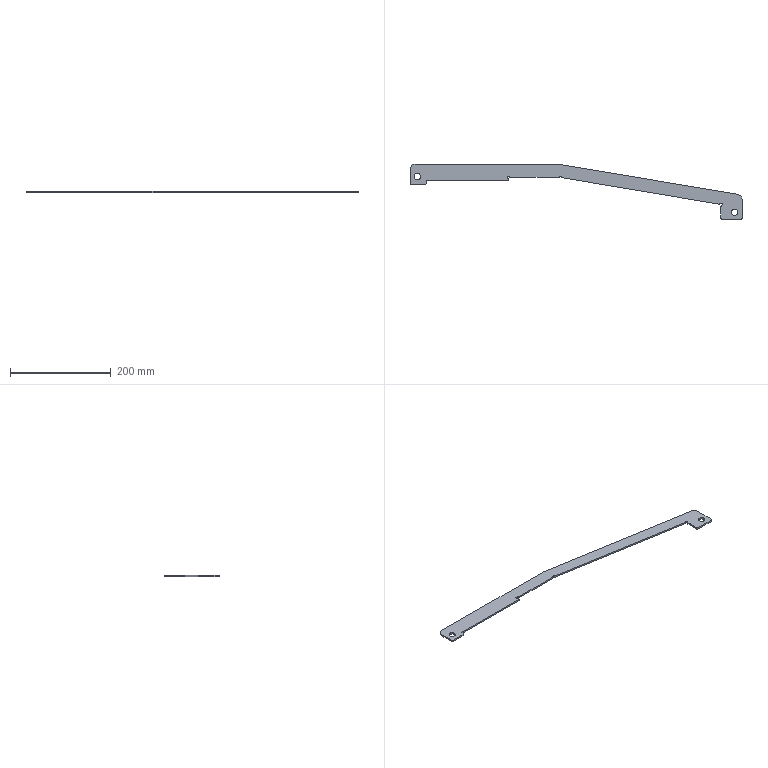Part | SolidWorks | features Fillet 2, FlatPattern 1, SMBaseFlange 1, SheetMetal 1 | 1 solid | 34 faces | box 659 x 110.2 x 3 mm | volume 58163 mm3 | cylinder 20 | plane 14 | commonest cylinder face diameters 4 x6 5 x4 6 x4 12.5 x4 20 x2
STEP:
#1=CARTESIAN_POINT('',(-277.647,51.799,3.));
#2=VERTEX_POINT('',#1);
#3=CARTESIAN_POINT('',(-265.147,51.799,3.));
#4=VERTEX_POINT('',#3);
#5=CARTESIAN_POINT('',(-271.397,51.799,3.));
#6=DIRECTION('',(0.,0.,1.));
#7=DIRECTION('',(1.,0.,0.));
#8=AXIS2_PLACEMENT_3D('',#5,#6,#7);
#9=CIRCLE('',#8,6.25);
#10=EDGE_CURVE('',#2,#4,#9,.T.);
#11=ORIENTED_EDGE('',*,*,#10,.T.);
#12=CARTESIAN_POINT('',(-265.147,51.799,0.));
#13=VERTEX_POINT('',#12);
#14=CARTESIAN_POINT('',(-265.147,51.799,3.));
#15=DIRECTION('',(0.,0.,-1.));
#16=VECTOR('',#15,1000.);
#17=LINE('',#14,#16);
#18=EDGE_CURVE('',#4,#13,#17,.T.);
#19=ORIENTED_EDGE('',*,*,#18,.T.);
#20=CARTESIAN_POINT('',(-277.647,51.799,0.));
#21=VERTEX_POINT('',#20);
#22=CARTESIAN_POINT('',(-271.397,51.799,0.));
#23=DIRECTION('',(0.,0.,1.));
#24=DIRECTION('',(1.,0.,0.));
#25=AXIS2_PLACEMENT_3D('',#22,#23,#24);
#26=CIRCLE('',#25,6.25);
#27=EDGE_CURVE('',#21,#13,#26,.T.);
#28=ORIENTED_EDGE('',*,*,#27,.F.);
#29=CARTESIAN_POINT('',(-277.647,51.799,3.));
#30=DIRECTION('',(0.,0.,-1.));
#31=VECTOR('',#30,1000.);
#32=LINE('',#29,#31);
#33=EDGE_CURVE('',#2,#21,#32,.T.);
#34=ORIENTED_EDGE('',*,*,#33,.F.);
#35=EDGE_LOOP('',(#11,#19,#28,#34));
#36=FACE_OUTER_BOUND('',#35,.T.);
#37=CARTESIAN_POINT('',(-271.397,51.799,3.));
#38=DIRECTION('',(0.,0.,-1.));
#39=DIRECTION('',(-1.,0.,0.));
#40=AXIS2_PLACEMENT_3D('',#37,#38,#39);
#41=CYLINDRICAL_SURFACE('',#40,6.25);
#42=ADVANCED_FACE('',(#36),#41,.F.);
#43=CARTESIAN_POINT('',(352.353,-18.901,3.));
#44=VERTEX_POINT('',#43);
#45=CARTESIAN_POINT('',(364.853,-18.901,3.));
#46=VERTEX_POINT('',#45);
#47=CARTESIAN_POINT('',(358.603,-18.901,3.));
#48=DIRECTION('',(0.,0.,1.));
#49=DIRECTION('',(1.,0.,0.));
#50=AXIS2_PLACEMENT_3D('',#47,#48,#49);
#51=CIRCLE('',#50,6.25);
#52=EDGE_CURVE('',#44,#46,#51,.T.);
#53=ORIENTED_EDGE('',*,*,#52,.T.);
#54=CARTESIAN_POINT('',(364.853,-18.901,0.));
#55=VERTEX_POINT('',#54);
#56=CARTESIAN_POINT('',(364.853,-18.901,3.));
#57=DIRECTION('',(0.,0.,-1.));
#58=VECTOR('',#57,1000.);
#59=LINE('',#56,#58);
#60=EDGE_CURVE('',#46,#55,#59,.T.);
#61=ORIENTED_EDGE('',*,*,#60,.T.);
#62=CARTESIAN_POINT('',(352.353,-18.901,0.));
#63=VERTEX_POINT('',#62);
#64=CARTESIAN_POINT('',(358.603,-18.901,0.));
#65=DIRECTION('',(0.,0.,1.));
#66=DIRECTION('',(1.,0.,0.));
#67=AXIS2_PLACEMENT_3D('',#64,#65,#66);
#68=CIRCLE('',#67,6.25);
#69=EDGE_CURVE('',#63,#55,#68,.T.);
#70=ORIENTED_EDGE('',*,*,#69,.F.);
#71=CARTESIAN_POINT('',(352.353,-18.901,3.));
#72=DIRECTION('',(0.,0.,-1.));
#73=VECTOR('',#72,1000.);
#74=LINE('',#71,#73);
#75=EDGE_CURVE('',#44,#63,#74,.T.);
#76=ORIENTED_EDGE('',*,*,#75,.F.);
#77=EDGE_LOOP('',(#53,#61,#70,#76));
#78=FACE_OUTER_BOUND('',#77,.T.);
#79=CARTESIAN_POINT('',(358.603,-18.901,3.));
#80=DIRECTION('',(0.,0.,-1.));
#81=DIRECTION('',(-1.,0.,0.));
#82=AXIS2_PLACEMENT_3D('',#79,#80,#81);
#83=CYLINDRICAL_SURFACE('',#82,6.25);
#84=ADVANCED_FACE('',(#78),#83,.F.);
#85=CARTESIAN_POINT('',(-92.897,50.099,3.));
#86=VERTEX_POINT('',#85);
#87=CARTESIAN_POINT('',(-88.157,51.21,3.));
#88=VERTEX_POINT('',#87);
#89=CARTESIAN_POINT('',(-90.397,50.099,3.));
#90=DIRECTION('',(0.,0.,-1.));
#91=DIRECTION('',(1.,0.,0.));
#92=AXIS2_PLACEMENT_3D('',#89,#90,#91);
#93=CIRCLE('',#92,2.5);
#94=EDGE_CURVE('',#86,#88,#93,.T.);
#95=ORIENTED_EDGE('',*,*,#94,.F.);
#96=CARTESIAN_POINT('',(-92.897,50.099,0.));
#97=VERTEX_POINT('',#96);
#98=CARTESIAN_POINT('',(-92.897,50.099,3.));
#99=DIRECTION('',(0.,0.,-1.));
#100=VECTOR('',#99,1000.);
#101=LINE('',#98,#100);
#102=EDGE_CURVE('',#86,#97,#101,.T.);
#103=ORIENTED_EDGE('',*,*,#102,.T.);
#104=CARTESIAN_POINT('',(-88.157,51.21,0.));
#105=VERTEX_POINT('',#104);
#106=CARTESIAN_POINT('',(-90.397,50.099,0.));
#107=DIRECTION('',(0.,0.,-1.));
#108=DIRECTION('',(1.,0.,0.));
#109=AXIS2_PLACEMENT_3D('',#106,#107,#108);
#110=CIRCLE('',#109,2.5);
#111=EDGE_CURVE('',#97,#105,#110,.T.);
#112=ORIENTED_EDGE('',*,*,#111,.T.);
#113=CARTESIAN_POINT('',(-88.157,51.21,3.));
#114=DIRECTION('',(0.,0.,1.));
#115=VECTOR('',#114,1000.);
#116=LINE('',#113,#115);
#117=EDGE_CURVE('',#105,#88,#116,.T.);
#118=ORIENTED_EDGE('',*,*,#117,.T.);
#119=EDGE_LOOP('',(#95,#103,#112,#118));
#120=FACE_OUTER_BOUND('',#119,.T.);
#121=CARTESIAN_POINT('',(-90.397,50.099,3.));
#122=DIRECTION('',(0.,0.,-1.));
#123=DIRECTION('',(-1.,0.,0.));
#124=AXIS2_PLACEMENT_3D('',#121,#122,#123);
#125=CYLINDRICAL_SURFACE('',#124,2.5);
#126=ADVANCED_FACE('',(#120),#125,.F.);
#127=CARTESIAN_POINT('',(-90.397,43.499,3.));
#128=VERTEX_POINT('',#127);
#129=CARTESIAN_POINT('',(-90.397,46.068,3.));
#130=VERTEX_POINT('',#129);
#131=CARTESIAN_POINT('',(-90.397,47.599,3.));
#132=DIRECTION('',(0.,1.,0.));
#133=VECTOR('',#132,1000.);
#134=LINE('',#131,#133);
#135=EDGE_CURVE('',#128,#130,#134,.T.);
#136=ORIENTED_EDGE('',*,*,#135,.T.);
#137=CARTESIAN_POINT('',(-91.508,47.86,3.));
#138=VERTEX_POINT('',#137);
#139=CARTESIAN_POINT('',(-92.397,46.068,3.));
#140=DIRECTION('',(0.,0.,1.));
#141=DIRECTION('',(-1.,0.,0.));
#142=AXIS2_PLACEMENT_3D('',#139,#140,#141);
#143=CIRCLE('',#142,2.);
#144=EDGE_CURVE('',#130,#138,#143,.T.);
#145=ORIENTED_EDGE('',*,*,#144,.T.);
#146=CARTESIAN_POINT('',(-90.397,50.099,3.));
#147=DIRECTION('',(0.,0.,-1.));
#148=DIRECTION('',(1.,0.,0.));
#149=AXIS2_PLACEMENT_3D('',#146,#147,#148);
#150=CIRCLE('',#149,2.5);
#151=EDGE_CURVE('',#138,#86,#150,.T.);
#152=ORIENTED_EDGE('',*,*,#151,.T.);
#153=ORIENTED_EDGE('',*,*,#94,.T.);
#154=CARTESIAN_POINT('',(-86.365,50.099,3.));
#155=VERTEX_POINT('',#154);
#156=CARTESIAN_POINT('',(-86.365,52.099,3.));
#157=DIRECTION('',(0.,0.,1.));
#158=DIRECTION('',(-1.,0.,0.));
#159=AXIS2_PLACEMENT_3D('',#156,#157,#158);
#160=CIRCLE('',#159,2.);
#161=EDGE_CURVE('',#88,#155,#160,.T.);
#162=ORIENTED_EDGE('',*,*,#161,.T.);
#163=CARTESIAN_POINT('',(8.706,50.099,3.));
#164=VERTEX_POINT('',#163);
#165=CARTESIAN_POINT('',(10.237,50.099,3.));
#166=DIRECTION('',(1.,-0.000000002,0.));
#167=VECTOR('',#166,1000.);
#168=LINE('',#165,#167);
#169=EDGE_CURVE('',#155,#164,#168,.T.);
#170=ORIENTED_EDGE('',*,*,#169,.T.);
#171=CARTESIAN_POINT('',(10.497,51.21,3.));
#172=VERTEX_POINT('',#171);
#173=CARTESIAN_POINT('',(8.706,52.099,3.));
#174=DIRECTION('',(0.,0.,1.));
#175=DIRECTION('',(-1.,0.,0.));
#176=AXIS2_PLACEMENT_3D('',#173,#174,#175);
#177=CIRCLE('',#176,2.);
#178=EDGE_CURVE('',#164,#172,#177,.T.);
#179=ORIENTED_EDGE('',*,*,#178,.T.);
#180=CARTESIAN_POINT('',(15.13,50.824,3.));
#181=VERTEX_POINT('',#180);
#182=CARTESIAN_POINT('',(12.737,50.099,3.));
#183=DIRECTION('',(0.,0.,-1.));
#184=DIRECTION('',(1.,0.,0.));
#185=AXIS2_PLACEMENT_3D('',#182,#183,#184);
#186=CIRCLE('',#185,2.5);
#187=EDGE_CURVE('',#172,#181,#186,.T.);
#188=ORIENTED_EDGE('',*,*,#187,.T.);
#189=CARTESIAN_POINT('',(16.712,49.431,3.));
#190=VERTEX_POINT('',#189);
#191=CARTESIAN_POINT('',(17.044,51.403,3.));
#192=DIRECTION('',(0.,0.,1.));
#193=DIRECTION('',(-1.,0.,0.));
#194=AXIS2_PLACEMENT_3D('',#191,#192,#193);
#195=CIRCLE('',#194,2.);
#196=EDGE_CURVE('',#181,#190,#195,.T.);
#197=ORIENTED_EDGE('',*,*,#196,.T.);
#198=CARTESIAN_POINT('',(327.328,-2.779,3.));
#199=VERTEX_POINT('',#198);
#200=CARTESIAN_POINT('',(328.838,-3.033,3.));
#201=DIRECTION('',(0.9862,-0.1658,0.));
#202=VECTOR('',#201,1000.);
#203=LINE('',#200,#202);
#204=EDGE_CURVE('',#190,#199,#203,.T.);
#205=ORIENTED_EDGE('',*,*,#204,.T.);
#206=CARTESIAN_POINT('',(329.279,-1.98,3.));
#207=VERTEX_POINT('',#206);
#208=CARTESIAN_POINT('',(327.66,-0.8068,3.));
#209=DIRECTION('',(0.,0.,1.));
#210=DIRECTION('',(-1.,0.,0.));
#211=AXIS2_PLACEMENT_3D('',#208,#209,#210);
#212=CIRCLE('',#211,2.);
#213=EDGE_CURVE('',#199,#207,#212,.T.);
#214=ORIENTED_EDGE('',*,*,#213,.T.);
#215=CARTESIAN_POINT('',(332.415,-5.687,3.));
#216=VERTEX_POINT('',#215);
#217=CARTESIAN_POINT('',(331.303,-3.447,3.));
#218=DIRECTION('',(0.,0.,-1.));
#219=DIRECTION('',(1.,0.,0.));
#220=AXIS2_PLACEMENT_3D('',#217,#218,#219);
#221=CIRCLE('',#220,2.5);
#222=EDGE_CURVE('',#207,#216,#221,.T.);
#223=ORIENTED_EDGE('',*,*,#222,.T.);
#224=CARTESIAN_POINT('',(331.303,-7.478,3.));
#225=VERTEX_POINT('',#224);
#226=CARTESIAN_POINT('',(333.303,-7.478,3.));
#227=DIRECTION('',(0.,0.,1.));
#228=DIRECTION('',(-1.,0.,0.));
#229=AXIS2_PLACEMENT_3D('',#226,#227,#228);
#230=CIRCLE('',#229,2.);
#231=EDGE_CURVE('',#216,#225,#230,.T.);
#232=ORIENTED_EDGE('',*,*,#231,.T.);
#233=CARTESIAN_POINT('',(331.303,-30.901,3.));
#234=VERTEX_POINT('',#233);
#235=CARTESIAN_POINT('',(331.303,-33.901,3.));
#236=DIRECTION('',(0.,-1.,0.));
#237=VECTOR('',#236,1000.);
#238=LINE('',#235,#237);
#239=EDGE_CURVE('',#225,#234,#238,.T.);
#240=ORIENTED_EDGE('',*,*,#239,.T.);
#241=CARTESIAN_POINT('',(334.303,-33.901,3.));
#242=VERTEX_POINT('',#241);
#243=CARTESIAN_POINT('',(334.303,-30.901,3.));
#244=DIRECTION('',(0.,0.,1.));
#245=DIRECTION('',(-1.,0.,0.));
#246=AXIS2_PLACEMENT_3D('',#243,#244,#245);
#247=CIRCLE('',#246,3.);
#248=EDGE_CURVE('',#234,#242,#247,.T.);
#249=ORIENTED_EDGE('',*,*,#248,.T.);
#250=CARTESIAN_POINT('',(370.103,-33.901,3.));
#251=VERTEX_POINT('',#250);
#252=CARTESIAN_POINT('',(331.303,-33.901,3.));
#253=DIRECTION('',(1.,0.,0.));
#254=VECTOR('',#253,1000.);
#255=LINE('',#252,#254);
#256=EDGE_CURVE('',#242,#251,#255,.T.);
#257=ORIENTED_EDGE('',*,*,#256,.T.);
#258=CARTESIAN_POINT('',(373.103,-30.901,3.));
#259=VERTEX_POINT('',#258);
#260=CARTESIAN_POINT('',(370.103,-30.901,3.));
#261=DIRECTION('',(0.,0.,1.));
#262=DIRECTION('',(-1.,0.,0.));
#263=AXIS2_PLACEMENT_3D('',#260,#261,#262);
#264=CIRCLE('',#263,3.);
#265=EDGE_CURVE('',#251,#259,#264,.T.);
#266=ORIENTED_EDGE('',*,*,#265,.T.);
#267=CARTESIAN_POINT('',(373.103,6.871,3.));
#268=VERTEX_POINT('',#267);
#269=CARTESIAN_POINT('',(373.103,-33.901,3.));
#270=DIRECTION('',(0.,1.,0.));
#271=VECTOR('',#270,1000.);
#272=LINE('',#269,#271);
#273=EDGE_CURVE('',#259,#268,#272,.T.);
#274=ORIENTED_EDGE('',*,*,#273,.T.);
#275=CARTESIAN_POINT('',(364.753,16.734,3.));
#276=VERTEX_POINT('',#275);
#277=CARTESIAN_POINT('',(363.103,6.871,3.));
#278=DIRECTION('',(0.,0.,1.));
#279=DIRECTION('',(-1.,0.,0.));
#280=AXIS2_PLACEMENT_3D('',#277,#278,#279);
#281=CIRCLE('',#280,10.);
#282=EDGE_CURVE('',#268,#276,#281,.T.);
#283=ORIENTED_EDGE('',*,*,#282,.T.);
#284=CARTESIAN_POINT('',(8.534,76.299,3.));
#285=VERTEX_POINT('',#284);
#286=CARTESIAN_POINT('',(364.753,16.734,3.));
#287=DIRECTION('',(-0.9863,0.1649,0.));
#288=VECTOR('',#287,1000.);
#289=LINE('',#286,#288);
#290=EDGE_CURVE('',#276,#285,#289,.T.);
#291=ORIENTED_EDGE('',*,*,#290,.T.);
#292=CARTESIAN_POINT('',(-275.897,76.299,3.));
#293=VERTEX_POINT('',#292);
#294=CARTESIAN_POINT('',(-275.897,76.299,3.));
#295=DIRECTION('',(-1.,0.,0.));
#296=VECTOR('',#295,1000.);
#297=LINE('',#294,#296);
#298=EDGE_CURVE('',#285,#293,#297,.T.);
#299=ORIENTED_EDGE('',*,*,#298,.T.);
#300=CARTESIAN_POINT('',(-285.897,66.299,3.));
#301=VERTEX_POINT('',#300);
#302=CARTESIAN_POINT('',(-275.897,66.299,3.));
#303=DIRECTION('',(0.,0.,1.));
#304=DIRECTION('',(-1.,0.,0.));
#305=AXIS2_PLACEMENT_3D('',#302,#303,#304);
#306=CIRCLE('',#305,10.);
#307=EDGE_CURVE('',#293,#301,#306,.T.);
#308=ORIENTED_EDGE('',*,*,#307,.T.);
#309=CARTESIAN_POINT('',(-285.897,39.299,3.));
#310=VERTEX_POINT('',#309);
#311=CARTESIAN_POINT('',(-285.897,36.299,3.));
#312=DIRECTION('',(0.,-1.,0.));
#313=VECTOR('',#312,1000.);
#314=LINE('',#311,#313);
#315=EDGE_CURVE('',#301,#310,#314,.T.);
#316=ORIENTED_EDGE('',*,*,#315,.T.);
#317=CARTESIAN_POINT('',(-282.897,36.299,3.));
#318=VERTEX_POINT('',#317);
#319=CARTESIAN_POINT('',(-282.897,39.299,3.));
#320=DIRECTION('',(0.,0.,1.));
#321=DIRECTION('',(-1.,0.,0.));
#322=AXIS2_PLACEMENT_3D('',#319,#320,#321);
#323=CIRCLE('',#322,3.);
#324=EDGE_CURVE('',#310,#318,#323,.T.);
#325=ORIENTED_EDGE('',*,*,#324,.T.);
#326=CARTESIAN_POINT('',(-256.397,36.299,3.));
#327=VERTEX_POINT('',#326);
#328=CARTESIAN_POINT('',(-253.397,36.299,3.));
#329=DIRECTION('',(1.,0.,0.));
#330=VECTOR('',#329,1000.);
#331=LINE('',#328,#330);
#332=EDGE_CURVE('',#318,#327,#331,.T.);
#333=ORIENTED_EDGE('',*,*,#332,.T.);
#334=CARTESIAN_POINT('',(-253.397,39.299,3.));
#335=VERTEX_POINT('',#334);
#336=CARTESIAN_POINT('',(-256.397,39.299,3.));
#337=DIRECTION('',(0.,0.,1.));
#338=DIRECTION('',(-1.,0.,0.));
#339=AXIS2_PLACEMENT_3D('',#336,#337,#338);
#340=CIRCLE('',#339,3.);
#341=EDGE_CURVE('',#327,#335,#340,.T.);
#342=ORIENTED_EDGE('',*,*,#341,.T.);
#343=CARTESIAN_POINT('',(-253.397,43.499,3.));
#344=VERTEX_POINT('',#343);
#345=CARTESIAN_POINT('',(-253.397,43.499,3.));
#346=DIRECTION('',(0.,1.,0.));
#347=VECTOR('',#346,1000.);
#348=LINE('',#345,#347);
#349=EDGE_CURVE('',#335,#344,#348,.T.);
#350=ORIENTED_EDGE('',*,*,#349,.T.);
#351=CARTESIAN_POINT('',(-90.397,43.499,3.));
#352=DIRECTION('',(1.,0.,0.));
#353=VECTOR('',#352,1000.);
#354=LINE('',#351,#353);
#355=EDGE_CURVE('',#344,#128,#354,.T.);
#356=ORIENTED_EDGE('',*,*,#355,.T.);
#357=EDGE_LOOP('',(#136,#145,#152,#153,#162,#170,#179,#188,#197,#205,#214,#223,#232,#240,#249,#257,#266,#274,#283,#291,#299,#308,#316,#325,#333,#342,#350,#356));
#358=FACE_OUTER_BOUND('',#357,.T.);
#359=ORIENTED_EDGE('',*,*,#52,.F.);
#360=CARTESIAN_POINT('',(358.603,-18.901,3.));
#361=DIRECTION('',(0.,0.,1.));
#362=DIRECTION('',(1.,0.,0.));
#363=AXIS2_PLACEMENT_3D('',#360,#361,#362);
#364=CIRCLE('',#363,6.25);
#365=EDGE_CURVE('',#46,#44,#364,.T.);
#366=ORIENTED_EDGE('',*,*,#365,.F.);
#367=EDGE_LOOP('',(#359,#366));
#368=FACE_BOUND('',#367,.T.);
#369=ORIENTED_EDGE('',*,*,#10,.F.);
#370=CARTESIAN_POINT('',(-271.397,51.799,3.));
#371=DIRECTION('',(0.,0.,1.));
#372=DIRECTION('',(1.,0.,0.));
#373=AXIS2_PLACEMENT_3D('',#370,#371,#372);
#374=CIRCLE('',#373,6.25);
#375=EDGE_CURVE('',#4,#2,#374,.T.);
#376=ORIENTED_EDGE('',*,*,#375,.F.);
#377=EDGE_LOOP('',(#369,#376));
#378=FACE_BOUND('',#377,.T.);
#379=CARTESIAN_POINT('',(-275.897,66.299,3.));
#380=DIRECTION('',(0.,0.,-1.));
#381=DIRECTION('',(-1.,0.,0.));
#382=AXIS2_PLACEMENT_3D('',#379,#380,#381);
#383=PLANE('',#382);
#384=ADVANCED_FACE('',(#358,#368,#378),#383,.F.);
#385=ORIENTED_EDGE('',*,*,#69,.T.);
#386=CARTESIAN_POINT('',(358.603,-18.901,0.));
#387=DIRECTION('',(0.,0.,1.));
#388=DIRECTION('',(1.,0.,0.));
#389=AXIS2_PLACEMENT_3D('',#386,#387,#388);
#390=CIRCLE('',#389,6.25);
#391=EDGE_CURVE('',#55,#63,#390,.T.);
#392=ORIENTED_EDGE('',*,*,#391,.T.);
#393=EDGE_LOOP('',(#385,#392));
#394=FACE_BOUND('',#393,.T.);
#395=CARTESIAN_POINT('',(-91.508,47.86,0.));
#396=VERTEX_POINT('',#395);
#397=CARTESIAN_POINT('',(-90.397,50.099,0.));
#398=DIRECTION('',(0.,0.,-1.));
#399=DIRECTION('',(1.,0.,0.));
#400=AXIS2_PLACEMENT_3D('',#397,#398,#399);
#401=CIRCLE('',#400,2.5);
#402=EDGE_CURVE('',#396,#97,#401,.T.);
#403=ORIENTED_EDGE('',*,*,#402,.F.);
#404=CARTESIAN_POINT('',(-90.397,46.068,0.));
#405=VERTEX_POINT('',#404);
#406=CARTESIAN_POINT('',(-92.397,46.068,0.));
#407=DIRECTION('',(0.,0.,-1.));
#408=DIRECTION('',(-1.,0.,0.));
#409=AXIS2_PLACEMENT_3D('',#406,#407,#408);
#410=CIRCLE('',#409,2.);
#411=EDGE_CURVE('',#396,#405,#410,.T.);
#412=ORIENTED_EDGE('',*,*,#411,.T.);
#413=CARTESIAN_POINT('',(-90.397,43.499,0.));
#414=VERTEX_POINT('',#413);
#415=CARTESIAN_POINT('',(-90.397,47.599,0.));
#416=DIRECTION('',(0.,1.,0.));
#417=VECTOR('',#416,1000.);
#418=LINE('',#415,#417);
#419=EDGE_CURVE('',#414,#405,#418,.T.);
#420=ORIENTED_EDGE('',*,*,#419,.F.);
#421=CARTESIAN_POINT('',(-253.397,43.499,0.));
#422=VERTEX_POINT('',#421);
#423=CARTESIAN_POINT('',(-90.397,43.499,0.));
#424=DIRECTION('',(1.,0.,0.));
#425=VECTOR('',#424,1000.);
#426=LINE('',#423,#425);
#427=EDGE_CURVE('',#422,#414,#426,.T.);
#428=ORIENTED_EDGE('',*,*,#427,.F.);
#429=CARTESIAN_POINT('',(-253.397,39.299,0.));
#430=VERTEX_POINT('',#429);
#431=CARTESIAN_POINT('',(-253.397,43.499,0.));
#432=DIRECTION('',(0.,1.,0.));
#433=VECTOR('',#432,1000.);
#434=LINE('',#431,#433);
#435=EDGE_CURVE('',#430,#422,#434,.T.);
#436=ORIENTED_EDGE('',*,*,#435,.F.);
#437=CARTESIAN_POINT('',(-256.397,36.299,0.));
#438=VERTEX_POINT('',#437);
#439=CARTESIAN_POINT('',(-256.397,39.299,0.));
#440=DIRECTION('',(0.,0.,-1.));
#441=DIRECTION('',(-1.,0.,0.));
#442=AXIS2_PLACEMENT_3D('',#439,#440,#441);
#443=CIRCLE('',#442,3.);
#444=EDGE_CURVE('',#430,#438,#443,.T.);
#445=ORIENTED_EDGE('',*,*,#444,.T.);
#446=CARTESIAN_POINT('',(-282.897,36.299,0.));
#447=VERTEX_POINT('',#446);
#448=CARTESIAN_POINT('',(-253.397,36.299,0.));
#449=DIRECTION('',(1.,0.,0.));
#450=VECTOR('',#449,1000.);
#451=LINE('',#448,#450);
#452=EDGE_CURVE('',#447,#438,#451,.T.);
#453=ORIENTED_EDGE('',*,*,#452,.F.);
#454=CARTESIAN_POINT('',(-285.897,39.299,0.));
#455=VERTEX_POINT('',#454);
#456=CARTESIAN_POINT('',(-282.897,39.299,0.));
#457=DIRECTION('',(0.,0.,-1.));
#458=DIRECTION('',(-1.,0.,0.));
#459=AXIS2_PLACEMENT_3D('',#456,#457,#458);
#460=CIRCLE('',#459,3.);
#461=EDGE_CURVE('',#447,#455,#460,.T.);
#462=ORIENTED_EDGE('',*,*,#461,.T.);
#463=CARTESIAN_POINT('',(-285.897,66.299,0.));
#464=VERTEX_POINT('',#463);
#465=CARTESIAN_POINT('',(-285.897,36.299,0.));
#466=DIRECTION('',(0.,-1.,0.));
#467=VECTOR('',#466,1000.);
#468=LINE('',#465,#467);
#469=EDGE_CURVE('',#464,#455,#468,.T.);
#470=ORIENTED_EDGE('',*,*,#469,.F.);
#471=CARTESIAN_POINT('',(-275.897,76.299,0.));
#472=VERTEX_POINT('',#471);
#473=CARTESIAN_POINT('',(-275.897,66.299,0.));
#474=DIRECTION('',(0.,0.,1.));
#475=DIRECTION('',(-1.,0.,0.));
#476=AXIS2_PLACEMENT_3D('',#473,#474,#475);
#477=CIRCLE('',#476,10.);
#478=EDGE_CURVE('',#472,#464,#477,.T.);
#479=ORIENTED_EDGE('',*,*,#478,.F.);
#480=CARTESIAN_POINT('',(8.534,76.299,0.));
#481=VERTEX_POINT('',#480);
#482=CARTESIAN_POINT('',(-275.897,76.299,0.));
#483=DIRECTION('',(-1.,0.,0.));
#484=VECTOR('',#483,1000.);
#485=LINE('',#482,#484);
#486=EDGE_CURVE('',#481,#472,#485,.T.);
#487=ORIENTED_EDGE('',*,*,#486,.F.);
#488=CARTESIAN_POINT('',(364.753,16.734,0.));
#489=VERTEX_POINT('',#488);
#490=CARTESIAN_POINT('',(364.753,16.734,0.));
#491=DIRECTION('',(-0.9863,0.1649,0.));
#492=VECTOR('',#491,1000.);
#493=LINE('',#490,#492);
#494=EDGE_CURVE('',#489,#481,#493,.T.);
#495=ORIENTED_EDGE('',*,*,#494,.F.);
#496=CARTESIAN_POINT('',(373.103,6.871,0.));
#497=VERTEX_POINT('',#496);
#498=CARTESIAN_POINT('',(363.103,6.871,0.));
#499=DIRECTION('',(0.,0.,1.));
#500=DIRECTION('',(-1.,0.,0.));
#501=AXIS2_PLACEMENT_3D('',#498,#499,#500);
#502=CIRCLE('',#501,10.);
#503=EDGE_CURVE('',#497,#489,#502,.T.);
#504=ORIENTED_EDGE('',*,*,#503,.F.);
#505=CARTESIAN_POINT('',(373.103,-30.901,0.));
#506=VERTEX_POINT('',#505);
#507=CARTESIAN_POINT('',(373.103,-33.901,0.));
#508=DIRECTION('',(0.,1.,0.));
#509=VECTOR('',#508,1000.);
#510=LINE('',#507,#509);
#511=EDGE_CURVE('',#506,#497,#510,.T.);
#512=ORIENTED_EDGE('',*,*,#511,.F.);
#513=CARTESIAN_POINT('',(370.103,-33.901,0.));
#514=VERTEX_POINT('',#513);
#515=CARTESIAN_POINT('',(370.103,-30.901,0.));
#516=DIRECTION('',(0.,0.,-1.));
#517=DIRECTION('',(-1.,0.,0.));
#518=AXIS2_PLACEMENT_3D('',#515,#516,#517);
#519=CIRCLE('',#518,3.);
#520=EDGE_CURVE('',#506,#514,#519,.T.);
#521=ORIENTED_EDGE('',*,*,#520,.T.);
#522=CARTESIAN_POINT('',(334.303,-33.901,0.));
#523=VERTEX_POINT('',#522);
#524=CARTESIAN_POINT('',(331.303,-33.901,0.));
#525=DIRECTION('',(1.,0.,0.));
#526=VECTOR('',#525,1000.);
#527=LINE('',#524,#526);
#528=EDGE_CURVE('',#523,#514,#527,.T.);
#529=ORIENTED_EDGE('',*,*,#528,.F.);
#530=CARTESIAN_POINT('',(331.303,-30.901,0.));
#531=VERTEX_POINT('',#530);
#532=CARTESIAN_POINT('',(334.303,-30.901,0.));
#533=DIRECTION('',(0.,0.,-1.));
#534=DIRECTION('',(-1.,0.,0.));
#535=AXIS2_PLACEMENT_3D('',#532,#533,#534);
#536=CIRCLE('',#535,3.);
#537=EDGE_CURVE('',#523,#531,#536,.T.);
#538=ORIENTED_EDGE('',*,*,#537,.T.);
#539=CARTESIAN_POINT('',(331.303,-7.478,0.));
#540=VERTEX_POINT('',#539);
#541=CARTESIAN_POINT('',(331.303,-33.901,0.));
#542=DIRECTION('',(0.,-1.,0.));
#543=VECTOR('',#542,1000.);
#544=LINE('',#541,#543);
#545=EDGE_CURVE('',#540,#531,#544,.T.);
#546=ORIENTED_EDGE('',*,*,#545,.F.);
#547=CARTESIAN_POINT('',(332.415,-5.687,0.));
#548=VERTEX_POINT('',#547);
#549=CARTESIAN_POINT('',(333.303,-7.478,0.));
#550=DIRECTION('',(0.,0.,-1.));
#551=DIRECTION('',(-1.,0.,0.));
#552=AXIS2_PLACEMENT_3D('',#549,#550,#551);
#553=CIRCLE('',#552,2.);
#554=EDGE_CURVE('',#540,#548,#553,.T.);
#555=ORIENTED_EDGE('',*,*,#554,.T.);
#556=CARTESIAN_POINT('',(329.279,-1.98,0.));
#557=VERTEX_POINT('',#556);
#558=CARTESIAN_POINT('',(331.303,-3.447,0.));
#559=DIRECTION('',(0.,0.,-1.));
#560=DIRECTION('',(1.,0.,0.));
#561=AXIS2_PLACEMENT_3D('',#558,#559,#560);
#562=CIRCLE('',#561,2.5);
#563=EDGE_CURVE('',#557,#548,#562,.T.);
#564=ORIENTED_EDGE('',*,*,#563,.F.);
#565=CARTESIAN_POINT('',(327.328,-2.779,0.));
#566=VERTEX_POINT('',#565);
#567=CARTESIAN_POINT('',(327.66,-0.8068,0.));
#568=DIRECTION('',(0.,0.,-1.));
#569=DIRECTION('',(-1.,0.,0.));
#570=AXIS2_PLACEMENT_3D('',#567,#568,#569);
#571=CIRCLE('',#570,2.);
#572=EDGE_CURVE('',#557,#566,#571,.T.);
#573=ORIENTED_EDGE('',*,*,#572,.T.);
#574=CARTESIAN_POINT('',(16.712,49.431,0.));
#575=VERTEX_POINT('',#574);
#576=CARTESIAN_POINT('',(328.838,-3.033,0.));
#577=DIRECTION('',(0.9862,-0.1658,0.));
#578=VECTOR('',#577,1000.);
#579=LINE('',#576,#578);
#580=EDGE_CURVE('',#575,#566,#579,.T.);
#581=ORIENTED_EDGE('',*,*,#580,.F.);
#582=CARTESIAN_POINT('',(15.13,50.824,0.));
#583=VERTEX_POINT('',#582);
#584=CARTESIAN_POINT('',(17.044,51.403,0.));
#585=DIRECTION('',(0.,0.,-1.));
#586=DIRECTION('',(-1.,0.,0.));
#587=AXIS2_PLACEMENT_3D('',#584,#585,#586);
#588=CIRCLE('',#587,2.);
#589=EDGE_CURVE('',#575,#583,#588,.T.);
#590=ORIENTED_EDGE('',*,*,#589,.T.);
#591=CARTESIAN_POINT('',(10.497,51.21,0.));
#592=VERTEX_POINT('',#591);
#593=CARTESIAN_POINT('',(12.737,50.099,0.));
#594=DIRECTION('',(0.,0.,-1.));
#595=DIRECTION('',(1.,0.,0.));
#596=AXIS2_PLACEMENT_3D('',#593,#594,#595);
#597=CIRCLE('',#596,2.5);
#598=EDGE_CURVE('',#592,#583,#597,.T.);
#599=ORIENTED_EDGE('',*,*,#598,.F.);
#600=CARTESIAN_POINT('',(8.706,50.099,0.));
#601=VERTEX_POINT('',#600);
#602=CARTESIAN_POINT('',(8.706,52.099,0.));
#603=DIRECTION('',(0.,0.,-1.));
#604=DIRECTION('',(-1.,0.,0.));
#605=AXIS2_PLACEMENT_3D('',#602,#603,#604);
#606=CIRCLE('',#605,2.);
#607=EDGE_CURVE('',#592,#601,#606,.T.);
#608=ORIENTED_EDGE('',*,*,#607,.T.);
#609=CARTESIAN_POINT('',(-86.365,50.099,0.));
#610=VERTEX_POINT('',#609);
#611=CARTESIAN_POINT('',(10.237,50.099,0.));
#612=DIRECTION('',(1.,-0.000000002,0.));
#613=VECTOR('',#612,1000.);
#614=LINE('',#611,#613);
#615=EDGE_CURVE('',#610,#601,#614,.T.);
#616=ORIENTED_EDGE('',*,*,#615,.F.);
#617=CARTESIAN_POINT('',(-86.365,52.099,0.));
#618=DIRECTION('',(0.,0.,-1.));
#619=DIRECTION('',(-1.,0.,0.));
#620=AXIS2_PLACEMENT_3D('',#617,#618,#619);
#621=CIRCLE('',#620,2.);
#622=EDGE_CURVE('',#610,#105,#621,.T.);
#623=ORIENTED_EDGE('',*,*,#622,.T.);
#624=ORIENTED_EDGE('',*,*,#111,.F.);
#625=EDGE_LOOP('',(#403,#412,#420,#428,#436,#445,#453,#462,#470,#479,#487,#495,#504,#512,#521,#529,#538,#546,#555,#564,#573,#581,#590,#599,#608,#616,#623,#624));
#626=FACE_OUTER_BOUND('',#625,.T.);
#627=ORIENTED_EDGE('',*,*,#27,.T.);
#628=CARTESIAN_POINT('',(-271.397,51.799,0.));
#629=DIRECTION('',(0.,0.,1.));
#630=DIRECTION('',(1.,0.,0.));
#631=AXIS2_PLACEMENT_3D('',#628,#629,#630);
#632=CIRCLE('',#631,6.25);
#633=EDGE_CURVE('',#13,#21,#632,.T.);
#634=ORIENTED_EDGE('',*,*,#633,.T.);
#635=EDGE_LOOP('',(#627,#634));
#636=FACE_BOUND('',#635,.T.);
#637=CARTESIAN_POINT('',(-275.897,66.299,0.));
#638=DIRECTION('',(0.,0.,-1.));
#639=DIRECTION('',(-1.,0.,0.));
#640=AXIS2_PLACEMENT_3D('',#637,#638,#639);
#641=PLANE('',#640);
#642=ADVANCED_FACE('',(#394,#626,#636),#641,.T.);
#643=ORIENTED_EDGE('',*,*,#419,.T.);
#644=CARTESIAN_POINT('',(-90.397,46.068,3.));
#645=DIRECTION('',(0.,0.,1.));
#646=VECTOR('',#645,1000.);
#647=LINE('',#644,#646);
#648=EDGE_CURVE('',#405,#130,#647,.T.);
#649=ORIENTED_EDGE('',*,*,#648,.T.);
#650=ORIENTED_EDGE('',*,*,#135,.F.);
#651=CARTESIAN_POINT('',(-90.397,43.499,3.));
#652=DIRECTION('',(0.,0.,-1.));
#653=VECTOR('',#652,1000.);
#654=LINE('',#651,#653);
#655=EDGE_CURVE('',#128,#414,#654,.T.);
#656=ORIENTED_EDGE('',*,*,#655,.T.);
#657=EDGE_LOOP('',(#643,#649,#650,#656));
#658=FACE_OUTER_BOUND('',#657,.T.);
#659=CARTESIAN_POINT('',(-90.397,47.599,3.));
#660=DIRECTION('',(-1.,0.,0.));
#661=DIRECTION('',(0.,-1.,0.));
#662=AXIS2_PLACEMENT_3D('',#659,#660,#661);
#663=PLANE('',#662);
#664=ADVANCED_FACE('',(#658),#663,.F.);
#665=ORIENTED_EDGE('',*,*,#102,.F.);
#666=ORIENTED_EDGE('',*,*,#151,.F.);
#667=CARTESIAN_POINT('',(-91.508,47.86,3.));
#668=DIRECTION('',(0.,0.,-1.));
#669=VECTOR('',#668,1000.);
#670=LINE('',#667,#669);
#671=EDGE_CURVE('',#138,#396,#670,.T.);
#672=ORIENTED_EDGE('',*,*,#671,.T.);
#673=ORIENTED_EDGE('',*,*,#402,.T.);
#674=EDGE_LOOP('',(#665,#666,#672,#673));
#675=FACE_OUTER_BOUND('',#674,.T.);
#676=CARTESIAN_POINT('',(-90.397,50.099,3.));
#677=DIRECTION('',(0.,0.,-1.));
#678=DIRECTION('',(-1.,0.,0.));
#679=AXIS2_PLACEMENT_3D('',#676,#677,#678);
#680=CYLINDRICAL_SURFACE('',#679,2.5);
#681=ADVANCED_FACE('',(#675),#680,.F.);
#682=ORIENTED_EDGE('',*,*,#169,.F.);
#683=CARTESIAN_POINT('',(-86.365,50.099,3.));
#684=DIRECTION('',(0.,0.,-1.));
#685=VECTOR('',#684,1000.);
#686=LINE('',#683,#685);
#687=EDGE_CURVE('',#155,#610,#686,.T.);
#688=ORIENTED_EDGE('',*,*,#687,.T.);
#689=ORIENTED_EDGE('',*,*,#615,.T.);
#690=CARTESIAN_POINT('',(8.706,50.099,3.));
#691=DIRECTION('',(0.,0.,1.));
#692=VECTOR('',#691,1000.);
#693=LINE('',#690,#692);
#694=EDGE_CURVE('',#601,#164,#693,.T.);
#695=ORIENTED_EDGE('',*,*,#694,.T.);
#696=EDGE_LOOP('',(#682,#688,#689,#695));
#697=FACE_OUTER_BOUND('',#696,.T.);
#698=CARTESIAN_POINT('',(10.237,50.099,3.));
#699=DIRECTION('',(0.000000002,1.,0.));
#700=DIRECTION('',(-1.,0.000000002,0.));
#701=AXIS2_PLACEMENT_3D('',#698,#699,#700);
#702=PLANE('',#701);
#703=ADVANCED_FACE('',(#697),#702,.F.);
#704=ORIENTED_EDGE('',*,*,#187,.F.);
#705=CARTESIAN_POINT('',(10.497,51.21,3.));
#706=DIRECTION('',(0.,0.,-1.));
#707=VECTOR('',#706,1000.);
#708=LINE('',#705,#707);
#709=EDGE_CURVE('',#172,#592,#708,.T.);
#710=ORIENTED_EDGE('',*,*,#709,.T.);
#711=ORIENTED_EDGE('',*,*,#598,.T.);
#712=CARTESIAN_POINT('',(15.13,50.824,3.));
#713=DIRECTION('',(0.,0.,1.));
#714=VECTOR('',#713,1000.);
#715=LINE('',#712,#714);
#716=EDGE_CURVE('',#583,#181,#715,.T.);
#717=ORIENTED_EDGE('',*,*,#716,.T.);
#718=EDGE_LOOP('',(#704,#710,#711,#717));
#719=FACE_OUTER_BOUND('',#718,.T.);
#720=CARTESIAN_POINT('',(12.737,50.099,3.));
#721=DIRECTION('',(0.,0.,-1.));
#722=DIRECTION('',(-1.,0.,0.));
#723=AXIS2_PLACEMENT_3D('',#720,#721,#722);
#724=CYLINDRICAL_SURFACE('',#723,2.5);
#725=ADVANCED_FACE('',(#719),#724,.F.);
#726=ORIENTED_EDGE('',*,*,#204,.F.);
#727=CARTESIAN_POINT('',(16.712,49.431,3.));
#728=DIRECTION('',(0.,0.,-1.));
#729=VECTOR('',#728,1000.);
#730=LINE('',#727,#729);
#731=EDGE_CURVE('',#190,#575,#730,.T.);
#732=ORIENTED_EDGE('',*,*,#731,.T.);
#733=ORIENTED_EDGE('',*,*,#580,.T.);
#734=CARTESIAN_POINT('',(327.328,-2.779,3.));
#735=DIRECTION('',(0.,0.,1.));
#736=VECTOR('',#735,1000.);
#737=LINE('',#734,#736);
#738=EDGE_CURVE('',#566,#199,#737,.T.);
#739=ORIENTED_EDGE('',*,*,#738,.T.);
#740=EDGE_LOOP('',(#726,#732,#733,#739));
#741=FACE_OUTER_BOUND('',#740,.T.);
#742=CARTESIAN_POINT('',(328.838,-3.033,3.));
#743=DIRECTION('',(0.1658,0.9862,0.));
#744=DIRECTION('',(-0.9862,0.1658,0.));
#745=AXIS2_PLACEMENT_3D('',#742,#743,#744);
#746=PLANE('',#745);
#747=ADVANCED_FACE('',(#741),#746,.F.);
#748=ORIENTED_EDGE('',*,*,#563,.T.);
#749=CARTESIAN_POINT('',(332.415,-5.687,3.));
#750=DIRECTION('',(0.,0.,1.));
#751=VECTOR('',#750,1000.);
#752=LINE('',#749,#751);
#753=EDGE_CURVE('',#548,#216,#752,.T.);
#754=ORIENTED_EDGE('',*,*,#753,.T.);
#755=ORIENTED_EDGE('',*,*,#222,.F.);
#756=CARTESIAN_POINT('',(329.279,-1.98,3.));
#757=DIRECTION('',(0.,0.,-1.));
#758=VECTOR('',#757,1000.);
#759=LINE('',#756,#758);
#760=EDGE_CURVE('',#207,#557,#759,.T.);
#761=ORIENTED_EDGE('',*,*,#760,.T.);
#762=EDGE_LOOP('',(#748,#754,#755,#761));
#763=FACE_OUTER_BOUND('',#762,.T.);
#764=CARTESIAN_POINT('',(331.303,-3.447,3.));
#765=DIRECTION('',(0.,0.,-1.));
#766=DIRECTION('',(-1.,0.,0.));
#767=AXIS2_PLACEMENT_3D('',#764,#765,#766);
#768=CYLINDRICAL_SURFACE('',#767,2.5);
#769=ADVANCED_FACE('',(#763),#768,.F.);
#770=ORIENTED_EDGE('',*,*,#239,.F.);
#771=CARTESIAN_POINT('',(331.303,-7.478,3.));
#772=DIRECTION('',(0.,0.,-1.));
#773=VECTOR('',#772,1000.);
#774=LINE('',#771,#773);
#775=EDGE_CURVE('',#225,#540,#774,.T.);
#776=ORIENTED_EDGE('',*,*,#775,.T.);
#777=ORIENTED_EDGE('',*,*,#545,.T.);
#778=CARTESIAN_POINT('',(331.303,-30.901,3.));
#779=DIRECTION('',(0.,0.,1.));
#780=VECTOR('',#779,1000.);
#781=LINE('',#778,#780);
#782=EDGE_CURVE('',#531,#234,#781,.T.);
#783=ORIENTED_EDGE('',*,*,#782,.T.);
#784=EDGE_LOOP('',(#770,#776,#777,#783));
#785=FACE_OUTER_BOUND('',#784,.T.);
#786=CARTESIAN_POINT('',(331.303,-33.901,3.));
#787=DIRECTION('',(1.,0.,0.));
#788=DIRECTION('',(0.,0.,-1.));
#789=AXIS2_PLACEMENT_3D('',#786,#787,#788);
#790=PLANE('',#789);
#791=ADVANCED_FACE('',(#785),#790,.F.);
#792=ORIENTED_EDGE('',*,*,#528,.T.);
#793=CARTESIAN_POINT('',(370.103,-33.901,3.));
#794=DIRECTION('',(0.,0.,1.));
#795=VECTOR('',#794,1000.);
#796=LINE('',#793,#795);
#797=EDGE_CURVE('',#514,#251,#796,.T.);
#798=ORIENTED_EDGE('',*,*,#797,.T.);
#799=ORIENTED_EDGE('',*,*,#256,.F.);
#800=CARTESIAN_POINT('',(334.303,-33.901,3.));
#801=DIRECTION('',(0.,0.,-1.));
#802=VECTOR('',#801,1000.);
#803=LINE('',#800,#802);
#804=EDGE_CURVE('',#242,#523,#803,.T.);
#805=ORIENTED_EDGE('',*,*,#804,.T.);
#806=EDGE_LOOP('',(#792,#798,#799,#805));
#807=FACE_OUTER_BOUND('',#806,.T.);
#808=CARTESIAN_POINT('',(331.303,-33.901,3.));
#809=DIRECTION('',(0.,1.,0.));
#810=DIRECTION('',(0.,0.,1.));
#811=AXIS2_PLACEMENT_3D('',#808,#809,#810);
#812=PLANE('',#811);
#813=ADVANCED_FACE('',(#807),#812,.F.);
#814=ORIENTED_EDGE('',*,*,#273,.F.);
#815=CARTESIAN_POINT('',(373.103,-30.901,3.));
#816=DIRECTION('',(0.,0.,-1.));
#817=VECTOR('',#816,1000.);
#818=LINE('',#815,#817);
#819=EDGE_CURVE('',#259,#506,#818,.T.);
#820=ORIENTED_EDGE('',*,*,#819,.T.);
#821=ORIENTED_EDGE('',*,*,#511,.T.);
#822=CARTESIAN_POINT('',(373.103,6.871,3.));
#823=DIRECTION('',(0.,0.,-1.));
#824=VECTOR('',#823,1000.);
#825=LINE('',#822,#824);
#826=EDGE_CURVE('',#268,#497,#825,.T.);
#827=ORIENTED_EDGE('',*,*,#826,.F.);
#828=EDGE_LOOP('',(#814,#820,#821,#827));
#829=FACE_OUTER_BOUND('',#828,.T.);
#830=CARTESIAN_POINT('',(373.103,-33.901,3.));
#831=DIRECTION('',(-1.,0.,0.));
#832=DIRECTION('',(0.,0.,1.));
#833=AXIS2_PLACEMENT_3D('',#830,#831,#832);
#834=PLANE('',#833);
#835=ADVANCED_FACE('',(#829),#834,.F.);
#836=ORIENTED_EDGE('',*,*,#503,.T.);
#837=CARTESIAN_POINT('',(364.753,16.734,3.));
#838=DIRECTION('',(0.,0.,-1.));
#839=VECTOR('',#838,1000.);
#840=LINE('',#837,#839);
#841=EDGE_CURVE('',#276,#489,#840,.T.);
#842=ORIENTED_EDGE('',*,*,#841,.F.);
#843=ORIENTED_EDGE('',*,*,#282,.F.);
#844=ORIENTED_EDGE('',*,*,#826,.T.);
#845=EDGE_LOOP('',(#836,#842,#843,#844));
#846=FACE_OUTER_BOUND('',#845,.T.);
#847=CARTESIAN_POINT('',(363.103,6.871,3.));
#848=DIRECTION('',(0.,0.,-1.));
#849=DIRECTION('',(-1.,0.,0.));
#850=AXIS2_PLACEMENT_3D('',#847,#848,#849);
#851=CYLINDRICAL_SURFACE('',#850,10.);
#852=ADVANCED_FACE('',(#846),#851,.T.);
#853=ORIENTED_EDGE('',*,*,#494,.T.);
#854=CARTESIAN_POINT('',(8.534,76.299,3.));
#855=DIRECTION('',(0.,0.,-1.));
#856=VECTOR('',#855,1000.);
#857=LINE('',#854,#856);
#858=EDGE_CURVE('',#285,#481,#857,.T.);
#859=ORIENTED_EDGE('',*,*,#858,.F.);
#860=ORIENTED_EDGE('',*,*,#290,.F.);
#861=ORIENTED_EDGE('',*,*,#841,.T.);
#862=EDGE_LOOP('',(#853,#859,#860,#861));
#863=FACE_OUTER_BOUND('',#862,.T.);
#864=CARTESIAN_POINT('',(364.753,16.734,3.));
#865=DIRECTION('',(-0.1649,-0.9863,0.));
#866=DIRECTION('',(0.9863,-0.1649,0.));
#867=AXIS2_PLACEMENT_3D('',#864,#865,#866);
#868=PLANE('',#867);
#869=ADVANCED_FACE('',(#863),#868,.F.);
#870=ORIENTED_EDGE('',*,*,#486,.T.);
#871=CARTESIAN_POINT('',(-275.897,76.299,3.));
#872=DIRECTION('',(0.,0.,-1.));
#873=VECTOR('',#872,1000.);
#874=LINE('',#871,#873);
#875=EDGE_CURVE('',#293,#472,#874,.T.);
#876=ORIENTED_EDGE('',*,*,#875,.F.);
#877=ORIENTED_EDGE('',*,*,#298,.F.);
#878=ORIENTED_EDGE('',*,*,#858,.T.);
#879=EDGE_LOOP('',(#870,#876,#877,#878));
#880=FACE_OUTER_BOUND('',#879,.T.);
#881=CARTESIAN_POINT('',(-275.897,76.299,3.));
#882=DIRECTION('',(0.,-1.,0.));
#883=DIRECTION('',(0.,0.,-1.));
#884=AXIS2_PLACEMENT_3D('',#881,#882,#883);
#885=PLANE('',#884);
#886=ADVANCED_FACE('',(#880),#885,.F.);
#887=ORIENTED_EDGE('',*,*,#478,.T.);
#888=CARTESIAN_POINT('',(-285.897,66.299,3.));
#889=DIRECTION('',(0.,0.,-1.));
#890=VECTOR('',#889,1000.);
#891=LINE('',#888,#890);
#892=EDGE_CURVE('',#301,#464,#891,.T.);
#893=ORIENTED_EDGE('',*,*,#892,.F.);
#894=ORIENTED_EDGE('',*,*,#307,.F.);
#895=ORIENTED_EDGE('',*,*,#875,.T.);
#896=EDGE_LOOP('',(#887,#893,#894,#895));
#897=FACE_OUTER_BOUND('',#896,.T.);
#898=CARTESIAN_POINT('',(-275.897,66.299,3.));
#899=DIRECTION('',(0.,0.,-1.));
#900=DIRECTION('',(-1.,0.,0.));
#901=AXIS2_PLACEMENT_3D('',#898,#899,#900);
#902=CYLINDRICAL_SURFACE('',#901,10.);
#903=ADVANCED_FACE('',(#897),#902,.T.);
#904=ORIENTED_EDGE('',*,*,#469,.T.);
#905=CARTESIAN_POINT('',(-285.897,39.299,3.));
#906=DIRECTION('',(0.,0.,1.));
#907=VECTOR('',#906,1000.);
#908=LINE('',#905,#907);
#909=EDGE_CURVE('',#455,#310,#908,.T.);
#910=ORIENTED_EDGE('',*,*,#909,.T.);
#911=ORIENTED_EDGE('',*,*,#315,.F.);
#912=ORIENTED_EDGE('',*,*,#892,.T.);
#913=EDGE_LOOP('',(#904,#910,#911,#912));
#914=FACE_OUTER_BOUND('',#913,.T.);
#915=CARTESIAN_POINT('',(-285.897,36.299,3.));
#916=DIRECTION('',(1.,0.,0.));
#917=DIRECTION('',(0.,0.,-1.));
#918=AXIS2_PLACEMENT_3D('',#915,#916,#917);
#919=PLANE('',#918);
#920=ADVANCED_FACE('',(#914),#919,.F.);
#921=ORIENTED_EDGE('',*,*,#452,.T.);
#922=CARTESIAN_POINT('',(-256.397,36.299,3.));
#923=DIRECTION('',(0.,0.,1.));
#924=VECTOR('',#923,1000.);
#925=LINE('',#922,#924);
#926=EDGE_CURVE('',#438,#327,#925,.T.);
#927=ORIENTED_EDGE('',*,*,#926,.T.);
#928=ORIENTED_EDGE('',*,*,#332,.F.);
#929=CARTESIAN_POINT('',(-282.897,36.299,3.));
#930=DIRECTION('',(0.,0.,-1.));
#931=VECTOR('',#930,1000.);
#932=LINE('',#929,#931);
#933=EDGE_CURVE('',#318,#447,#932,.T.);
#934=ORIENTED_EDGE('',*,*,#933,.T.);
#935=EDGE_LOOP('',(#921,#927,#928,#934));
#936=FACE_OUTER_BOUND('',#935,.T.);
#937=CARTESIAN_POINT('',(-253.397,36.299,3.));
#938=DIRECTION('',(0.,1.,0.));
#939=DIRECTION('',(-1.,0.,0.));
#940=AXIS2_PLACEMENT_3D('',#937,#938,#939);
#941=PLANE('',#940);
#942=ADVANCED_FACE('',(#936),#941,.F.);
#943=ORIENTED_EDGE('',*,*,#349,.F.);
#944=CARTESIAN_POINT('',(-253.397,39.299,3.));
#945=DIRECTION('',(0.,0.,-1.));
#946=VECTOR('',#945,1000.);
#947=LINE('',#944,#946);
#948=EDGE_CURVE('',#335,#430,#947,.T.);
#949=ORIENTED_EDGE('',*,*,#948,.T.);
#950=ORIENTED_EDGE('',*,*,#435,.T.);
#951=CARTESIAN_POINT('',(-253.397,43.499,3.));
#952=DIRECTION('',(0.,0.,-1.));
#953=VECTOR('',#952,1000.);
#954=LINE('',#951,#953);
#955=EDGE_CURVE('',#344,#422,#954,.T.);
#956=ORIENTED_EDGE('',*,*,#955,.F.);
#957=EDGE_LOOP('',(#943,#949,#950,#956));
#958=FACE_OUTER_BOUND('',#957,.T.);
#959=CARTESIAN_POINT('',(-253.397,43.499,3.));
#960=DIRECTION('',(-1.,0.,0.));
#961=DIRECTION('',(0.,0.,1.));
#962=AXIS2_PLACEMENT_3D('',#959,#960,#961);
#963=PLANE('',#962);
#964=ADVANCED_FACE('',(#958),#963,.F.);
#965=ORIENTED_EDGE('',*,*,#427,.T.);
#966=ORIENTED_EDGE('',*,*,#655,.F.);
#967=ORIENTED_EDGE('',*,*,#355,.F.);
#968=ORIENTED_EDGE('',*,*,#955,.T.);
#969=EDGE_LOOP('',(#965,#966,#967,#968));
#970=FACE_OUTER_BOUND('',#969,.T.);
#971=CARTESIAN_POINT('',(-90.397,43.499,3.));
#972=DIRECTION('',(0.,1.,0.));
#973=DIRECTION('',(-1.,0.,0.));
#974=AXIS2_PLACEMENT_3D('',#971,#972,#973);
#975=PLANE('',#974);
#976=ADVANCED_FACE('',(#970),#975,.F.);
#977=ORIENTED_EDGE('',*,*,#60,.F.);
#978=ORIENTED_EDGE('',*,*,#365,.T.);
#979=ORIENTED_EDGE('',*,*,#75,.T.);
#980=ORIENTED_EDGE('',*,*,#391,.F.);
#981=EDGE_LOOP('',(#977,#978,#979,#980));
#982=FACE_OUTER_BOUND('',#981,.T.);
#983=CARTESIAN_POINT('',(358.603,-18.901,3.));
#984=DIRECTION('',(0.,0.,-1.));
#985=DIRECTION('',(-1.,0.,0.));
#986=AXIS2_PLACEMENT_3D('',#983,#984,#985);
#987=CYLINDRICAL_SURFACE('',#986,6.25);
#988=ADVANCED_FACE('',(#982),#987,.F.);
#989=ORIENTED_EDGE('',*,*,#18,.F.);
#990=ORIENTED_EDGE('',*,*,#375,.T.);
#991=ORIENTED_EDGE('',*,*,#33,.T.);
#992=ORIENTED_EDGE('',*,*,#633,.F.);
#993=EDGE_LOOP('',(#989,#990,#991,#992));
#994=FACE_OUTER_BOUND('',#993,.T.);
#995=CARTESIAN_POINT('',(-271.397,51.799,3.));
#996=DIRECTION('',(0.,0.,-1.));
#997=DIRECTION('',(-1.,0.,0.));
#998=AXIS2_PLACEMENT_3D('',#995,#996,#997);
#999=CYLINDRICAL_SURFACE('',#998,6.25);
#1000=ADVANCED_FACE('',(#994),#999,.F.);
#1001=ORIENTED_EDGE('',*,*,#265,.F.);
#1002=ORIENTED_EDGE('',*,*,#797,.F.);
#1003=ORIENTED_EDGE('',*,*,#520,.F.);
#1004=ORIENTED_EDGE('',*,*,#819,.F.);
#1005=EDGE_LOOP('',(#1001,#1002,#1003,#1004));
#1006=FACE_OUTER_BOUND('',#1005,.T.);
#1007=CARTESIAN_POINT('',(370.103,-30.901,3.));
#1008=DIRECTION('',(0.,0.,-1.));
#1009=DIRECTION('',(-1.,0.,0.));
#1010=AXIS2_PLACEMENT_3D('',#1007,#1008,#1009);
#1011=CYLINDRICAL_SURFACE('',#1010,3.);
#1012=ADVANCED_FACE('',(#1006),#1011,.T.);
#1013=ORIENTED_EDGE('',*,*,#248,.F.);
#1014=ORIENTED_EDGE('',*,*,#782,.F.);
#1015=ORIENTED_EDGE('',*,*,#537,.F.);
#1016=ORIENTED_EDGE('',*,*,#804,.F.);
#1017=EDGE_LOOP('',(#1013,#1014,#1015,#1016));
#1018=FACE_OUTER_BOUND('',#1017,.T.);
#1019=CARTESIAN_POINT('',(334.303,-30.901,3.));
#1020=DIRECTION('',(0.,0.,-1.));
#1021=DIRECTION('',(-1.,0.,0.));
#1022=AXIS2_PLACEMENT_3D('',#1019,#1020,#1021);
#1023=CYLINDRICAL_SURFACE('',#1022,3.);
#1024=ADVANCED_FACE('',(#1018),#1023,.T.);
#1025=ORIENTED_EDGE('',*,*,#341,.F.);
#1026=ORIENTED_EDGE('',*,*,#926,.F.);
#1027=ORIENTED_EDGE('',*,*,#444,.F.);
#1028=ORIENTED_EDGE('',*,*,#948,.F.);
#1029=EDGE_LOOP('',(#1025,#1026,#1027,#1028));
#1030=FACE_OUTER_BOUND('',#1029,.T.);
#1031=CARTESIAN_POINT('',(-256.397,39.299,3.));
#1032=DIRECTION('',(0.,0.,-1.));
#1033=DIRECTION('',(-1.,0.,0.));
#1034=AXIS2_PLACEMENT_3D('',#1031,#1032,#1033);
#1035=CYLINDRICAL_SURFACE('',#1034,3.);
#1036=ADVANCED_FACE('',(#1030),#1035,.T.);
#1037=ORIENTED_EDGE('',*,*,#324,.F.);
#1038=ORIENTED_EDGE('',*,*,#909,.F.);
#1039=ORIENTED_EDGE('',*,*,#461,.F.);
#1040=ORIENTED_EDGE('',*,*,#933,.F.);
#1041=EDGE_LOOP('',(#1037,#1038,#1039,#1040));
#1042=FACE_OUTER_BOUND('',#1041,.T.);
#1043=CARTESIAN_POINT('',(-282.897,39.299,3.));
#1044=DIRECTION('',(0.,0.,-1.));
#1045=DIRECTION('',(-1.,0.,0.));
#1046=AXIS2_PLACEMENT_3D('',#1043,#1044,#1045);
#1047=CYLINDRICAL_SURFACE('',#1046,3.);
#1048=ADVANCED_FACE('',(#1042),#1047,.T.);
#1049=ORIENTED_EDGE('',*,*,#144,.F.);
#1050=ORIENTED_EDGE('',*,*,#648,.F.);
#1051=ORIENTED_EDGE('',*,*,#411,.F.);
#1052=ORIENTED_EDGE('',*,*,#671,.F.);
#1053=EDGE_LOOP('',(#1049,#1050,#1051,#1052));
#1054=FACE_OUTER_BOUND('',#1053,.T.);
#1055=CARTESIAN_POINT('',(-92.397,46.068,3.));
#1056=DIRECTION('',(0.,0.,-1.));
#1057=DIRECTION('',(-1.,0.,0.));
#1058=AXIS2_PLACEMENT_3D('',#1055,#1056,#1057);
#1059=CYLINDRICAL_SURFACE('',#1058,2.);
#1060=ADVANCED_FACE('',(#1054),#1059,.T.);
#1061=ORIENTED_EDGE('',*,*,#161,.F.);
#1062=ORIENTED_EDGE('',*,*,#117,.F.);
#1063=ORIENTED_EDGE('',*,*,#622,.F.);
#1064=ORIENTED_EDGE('',*,*,#687,.F.);
#1065=EDGE_LOOP('',(#1061,#1062,#1063,#1064));
#1066=FACE_OUTER_BOUND('',#1065,.T.);
#1067=CARTESIAN_POINT('',(-86.365,52.099,3.));
#1068=DIRECTION('',(0.,0.,-1.));
#1069=DIRECTION('',(-1.,0.,0.));
#1070=AXIS2_PLACEMENT_3D('',#1067,#1068,#1069);
#1071=CYLINDRICAL_SURFACE('',#1070,2.);
#1072=ADVANCED_FACE('',(#1066),#1071,.T.);
#1073=ORIENTED_EDGE('',*,*,#178,.F.);
#1074=ORIENTED_EDGE('',*,*,#694,.F.);
#1075=ORIENTED_EDGE('',*,*,#607,.F.);
#1076=ORIENTED_EDGE('',*,*,#709,.F.);
#1077=EDGE_LOOP('',(#1073,#1074,#1075,#1076));
#1078=FACE_OUTER_BOUND('',#1077,.T.);
#1079=CARTESIAN_POINT('',(8.706,52.099,3.));
#1080=DIRECTION('',(0.,0.,-1.));
#1081=DIRECTION('',(-1.,0.,0.));
#1082=AXIS2_PLACEMENT_3D('',#1079,#1080,#1081);
#1083=CYLINDRICAL_SURFACE('',#1082,2.);
#1084=ADVANCED_FACE('',(#1078),#1083,.T.);
#1085=ORIENTED_EDGE('',*,*,#196,.F.);
#1086=ORIENTED_EDGE('',*,*,#716,.F.);
#1087=ORIENTED_EDGE('',*,*,#589,.F.);
#1088=ORIENTED_EDGE('',*,*,#731,.F.);
#1089=EDGE_LOOP('',(#1085,#1086,#1087,#1088));
#1090=FACE_OUTER_BOUND('',#1089,.T.);
#1091=CARTESIAN_POINT('',(17.044,51.403,3.));
#1092=DIRECTION('',(0.,0.,-1.));
#1093=DIRECTION('',(-1.,0.,0.));
#1094=AXIS2_PLACEMENT_3D('',#1091,#1092,#1093);
#1095=CYLINDRICAL_SURFACE('',#1094,2.);
#1096=ADVANCED_FACE('',(#1090),#1095,.T.);
#1097=ORIENTED_EDGE('',*,*,#231,.F.);
#1098=ORIENTED_EDGE('',*,*,#753,.F.);
#1099=ORIENTED_EDGE('',*,*,#554,.F.);
#1100=ORIENTED_EDGE('',*,*,#775,.F.);
#1101=EDGE_LOOP('',(#1097,#1098,#1099,#1100));
#1102=FACE_OUTER_BOUND('',#1101,.T.);
#1103=CARTESIAN_POINT('',(333.303,-7.478,3.));
#1104=DIRECTION('',(0.,0.,-1.));
#1105=DIRECTION('',(-1.,0.,0.));
#1106=AXIS2_PLACEMENT_3D('',#1103,#1104,#1105);
#1107=CYLINDRICAL_SURFACE('',#1106,2.);
#1108=ADVANCED_FACE('',(#1102),#1107,.T.);
#1109=ORIENTED_EDGE('',*,*,#213,.F.);
#1110=ORIENTED_EDGE('',*,*,#738,.F.);
#1111=ORIENTED_EDGE('',*,*,#572,.F.);
#1112=ORIENTED_EDGE('',*,*,#760,.F.);
#1113=EDGE_LOOP('',(#1109,#1110,#1111,#1112));
#1114=FACE_OUTER_BOUND('',#1113,.T.);
#1115=CARTESIAN_POINT('',(327.66,-0.8068,3.));
#1116=DIRECTION('',(0.,0.,-1.));
#1117=DIRECTION('',(-1.,0.,0.));
#1118=AXIS2_PLACEMENT_3D('',#1115,#1116,#1117);
#1119=CYLINDRICAL_SURFACE('',#1118,2.);
#1120=ADVANCED_FACE('',(#1114),#1119,.T.);
#1121=CLOSED_SHELL('',(#42,#84,#126,#384,#642,#664,#681,#703,#725,#747,#769,#791,#813,#835,#852,#869,#886,#903,#920,#942,#964,#976,#988,#1000,#1012,#1024,#1036,#1048,#1060,#1072,#1084,#1096,#1108,#1120));
#1122=MANIFOLD_SOLID_BREP('',#1121);
#1123=CARTESIAN_POINT('',(0.,0.,0.));
#1124=DIRECTION('',(0.,0.,1.));
#1125=DIRECTION('',(1.,0.,0.));
#1126=AXIS2_PLACEMENT_3D('',#1123,#1124,#1125);
#1127=(LENGTH_UNIT()NAMED_UNIT(*)SI_UNIT(.MILLI.,.METRE.));
#1128=UNCERTAINTY_MEASURE_WITH_UNIT(LENGTH_MEASURE(0.00001),#1127,'','');
#1129=(NAMED_UNIT(*)PLANE_ANGLE_UNIT()SI_UNIT($,.RADIAN.));
#1130=(NAMED_UNIT(*)SI_UNIT($,.STERADIAN.)SOLID_ANGLE_UNIT());
#1131=(GEOMETRIC_REPRESENTATION_CONTEXT(3)GLOBAL_UNCERTAINTY_ASSIGNED_CONTEXT((#1128))GLOBAL_UNIT_ASSIGNED_CONTEXT((#1127,#1129,#1130))REPRESENTATION_CONTEXT('',''));
#1132=ADVANCED_BREP_SHAPE_REPRESENTATION('',(#1122,#1126),#1131);